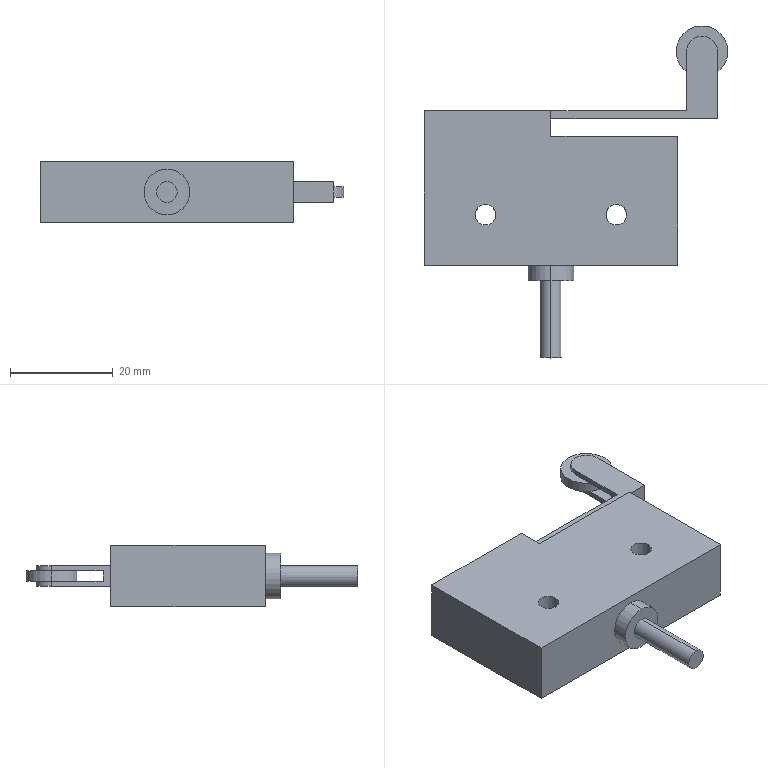Part | STEP file | Micro switch ZIR52-1703 | 2 solids | 32 faces | box 58.94 x 64.5 x 12 mm | volume 16845 mm3 | plane 20 | cylinder 12 | commonest cylinder face diameters 4 x6 6 x2 8.896 x2 10 x2